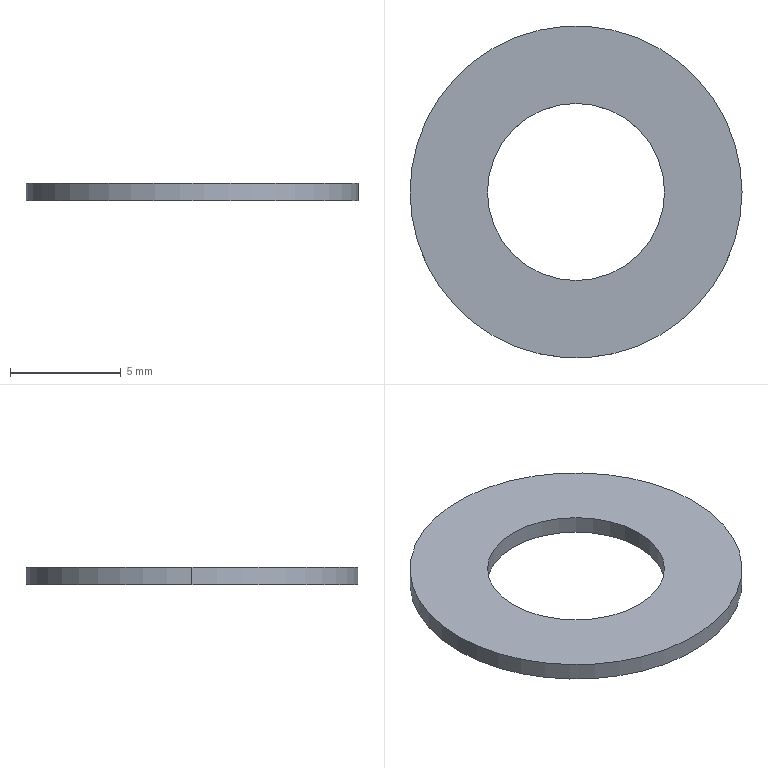Part | STEP file | E2E_X2D1_N_WASHER | 1 solid | 6 faces | box 15 x 15 x 0.8 mm | volume 101.159 mm3 | cylinder 4 | plane 2 | commonest cylinder face diameters 8 x2 15 x2
STEP:
#1=CARTESIAN_POINT('',(0.,0.,0.));
#2=DIRECTION('',(0.,0.,1.));
#3=DIRECTION('',(1.,0.,0.));
#4=AXIS2_PLACEMENT_3D('',#1,#2,#3);
#5=CARTESIAN_POINT('',(4.,0.,-0.8));
#6=VERTEX_POINT('',#5);
#7=CARTESIAN_POINT('',(4.,0.,0.));
#8=VERTEX_POINT('',#7);
#9=CARTESIAN_POINT('',(4.,0.,-0.8));
#10=DIRECTION('',(0.,0.,1.));
#11=VECTOR('',#10,1.);
#12=LINE('',#9,#11);
#13=CARTESIAN_POINT('',(0.,0.,-0.8));
#14=DIRECTION('',(0.,0.,1.));
#15=DIRECTION('',(1.,0.,0.));
#16=AXIS2_PLACEMENT_3D('',#13,#14,#15);
#17=CYLINDRICAL_SURFACE('',#16,4.);
#18=CARTESIAN_POINT('',(6.283,0.));
#19=DIRECTION('',(0.,1.));
#20=VECTOR('',#19,1.);
#21=LINE('',#18,#20);
#22=(GEOMETRIC_REPRESENTATION_CONTEXT(2)PARAMETRIC_REPRESENTATION_CONTEXT()REPRESENTATION_CONTEXT('',''));
#23=DEFINITIONAL_REPRESENTATION('',(#21),#22);
#24=PCURVE('',#17,#23);
#25=CARTESIAN_POINT('',(0.,0.,-0.8));
#26=DIRECTION('',(0.,0.,1.));
#27=DIRECTION('',(1.,0.,0.));
#28=AXIS2_PLACEMENT_3D('',#25,#26,#27);
#29=CYLINDRICAL_SURFACE('',#28,4.);
#30=CARTESIAN_POINT('',(0.,0.));
#31=DIRECTION('',(0.,1.));
#32=VECTOR('',#31,1.);
#33=LINE('',#30,#32);
#34=(GEOMETRIC_REPRESENTATION_CONTEXT(2)PARAMETRIC_REPRESENTATION_CONTEXT()REPRESENTATION_CONTEXT('',''));
#35=DEFINITIONAL_REPRESENTATION('',(#33),#34);
#36=PCURVE('',#29,#35);
#37=SURFACE_CURVE('',#12,(#24,#36),.PCURVE_S1.);
#38=EDGE_CURVE('',#6,#8,#37,.T.);
#39=ORIENTED_EDGE('',*,*,#38,.T.);
#40=CARTESIAN_POINT('',(-4.,0.,0.));
#41=VERTEX_POINT('',#40);
#42=CARTESIAN_POINT('',(0.,0.,0.));
#43=DIRECTION('',(0.,0.,1.));
#44=DIRECTION('',(1.,0.,0.));
#45=AXIS2_PLACEMENT_3D('',#42,#43,#44);
#46=CIRCLE('',#45,4.);
#47=CARTESIAN_POINT('',(0.,0.8));
#48=DIRECTION('',(1.,0.));
#49=VECTOR('',#48,1.);
#50=LINE('',#47,#49);
#51=(GEOMETRIC_REPRESENTATION_CONTEXT(2)PARAMETRIC_REPRESENTATION_CONTEXT()REPRESENTATION_CONTEXT('',''));
#52=DEFINITIONAL_REPRESENTATION('',(#50),#51);
#53=PCURVE('',#17,#52);
#54=CARTESIAN_POINT('',(0.,0.,0.));
#55=DIRECTION('',(0.,0.,1.));
#56=DIRECTION('',(1.,0.,0.));
#57=AXIS2_PLACEMENT_3D('',#54,#55,#56);
#58=PLANE('',#57);
#59=CARTESIAN_POINT('',(0.,0.));
#60=DIRECTION('',(1.,0.));
#61=AXIS2_PLACEMENT_2D('',#59,#60);
#62=CIRCLE('',#61,4.);
#63=(GEOMETRIC_REPRESENTATION_CONTEXT(2)PARAMETRIC_REPRESENTATION_CONTEXT()REPRESENTATION_CONTEXT('',''));
#64=DEFINITIONAL_REPRESENTATION('',(#62),#63);
#65=PCURVE('',#58,#64);
#66=SURFACE_CURVE('',#46,(#53,#65),.PCURVE_S1.);
#67=EDGE_CURVE('',#41,#8,#66,.T.);
#68=ORIENTED_EDGE('',*,*,#67,.F.);
#69=CARTESIAN_POINT('',(-4.,0.,-0.8));
#70=VERTEX_POINT('',#69);
#71=CARTESIAN_POINT('',(-4.,0.,-0.8));
#72=DIRECTION('',(0.,0.,1.));
#73=VECTOR('',#72,1.);
#74=LINE('',#71,#73);
#75=CARTESIAN_POINT('',(3.142,0.));
#76=DIRECTION('',(0.,1.));
#77=VECTOR('',#76,1.);
#78=LINE('',#75,#77);
#79=(GEOMETRIC_REPRESENTATION_CONTEXT(2)PARAMETRIC_REPRESENTATION_CONTEXT()REPRESENTATION_CONTEXT('',''));
#80=DEFINITIONAL_REPRESENTATION('',(#78),#79);
#81=PCURVE('',#17,#80);
#82=CARTESIAN_POINT('',(3.142,0.));
#83=DIRECTION('',(0.,1.));
#84=VECTOR('',#83,1.);
#85=LINE('',#82,#84);
#86=(GEOMETRIC_REPRESENTATION_CONTEXT(2)PARAMETRIC_REPRESENTATION_CONTEXT()REPRESENTATION_CONTEXT('',''));
#87=DEFINITIONAL_REPRESENTATION('',(#85),#86);
#88=PCURVE('',#29,#87);
#89=SURFACE_CURVE('',#74,(#81,#88),.PCURVE_S1.);
#90=EDGE_CURVE('',#70,#41,#89,.T.);
#91=ORIENTED_EDGE('',*,*,#90,.F.);
#92=CARTESIAN_POINT('',(0.,0.,-0.8));
#93=DIRECTION('',(0.,0.,1.));
#94=DIRECTION('',(1.,0.,0.));
#95=AXIS2_PLACEMENT_3D('',#92,#93,#94);
#96=CIRCLE('',#95,4.);
#97=CARTESIAN_POINT('',(0.,0.));
#98=DIRECTION('',(1.,0.));
#99=VECTOR('',#98,1.);
#100=LINE('',#97,#99);
#101=(GEOMETRIC_REPRESENTATION_CONTEXT(2)PARAMETRIC_REPRESENTATION_CONTEXT()REPRESENTATION_CONTEXT('',''));
#102=DEFINITIONAL_REPRESENTATION('',(#100),#101);
#103=PCURVE('',#17,#102);
#104=CARTESIAN_POINT('',(0.,0.,-0.8));
#105=DIRECTION('',(0.,0.,1.));
#106=DIRECTION('',(1.,0.,0.));
#107=AXIS2_PLACEMENT_3D('',#104,#105,#106);
#108=PLANE('',#107);
#109=CARTESIAN_POINT('',(0.,0.));
#110=DIRECTION('',(1.,0.));
#111=AXIS2_PLACEMENT_2D('',#109,#110);
#112=CIRCLE('',#111,4.);
#113=(GEOMETRIC_REPRESENTATION_CONTEXT(2)PARAMETRIC_REPRESENTATION_CONTEXT()REPRESENTATION_CONTEXT('',''));
#114=DEFINITIONAL_REPRESENTATION('',(#112),#113);
#115=PCURVE('',#108,#114);
#116=SURFACE_CURVE('',#96,(#103,#115),.PCURVE_S1.);
#117=EDGE_CURVE('',#70,#6,#116,.T.);
#118=ORIENTED_EDGE('',*,*,#117,.T.);
#119=EDGE_LOOP('',(#39,#68,#91,#118));
#120=FACE_BOUND('',#119,.F.);
#121=ADVANCED_FACE('',(#120),#17,.F.);
#122=CARTESIAN_POINT('',(7.5,0.,-0.8));
#123=VERTEX_POINT('',#122);
#124=CARTESIAN_POINT('',(-7.5,0.,-0.8));
#125=VERTEX_POINT('',#124);
#126=CARTESIAN_POINT('',(0.,0.,-0.8));
#127=DIRECTION('',(0.,0.,1.));
#128=DIRECTION('',(1.,0.,0.));
#129=AXIS2_PLACEMENT_3D('',#126,#127,#128);
#130=CIRCLE('',#129,7.5);
#131=CARTESIAN_POINT('',(0.,0.,-0.8));
#132=DIRECTION('',(0.,0.,1.));
#133=DIRECTION('',(1.,0.,0.));
#134=AXIS2_PLACEMENT_3D('',#131,#132,#133);
#135=CYLINDRICAL_SURFACE('',#134,7.5);
#136=CARTESIAN_POINT('',(0.,0.));
#137=DIRECTION('',(1.,0.));
#138=VECTOR('',#137,1.);
#139=LINE('',#136,#138);
#140=(GEOMETRIC_REPRESENTATION_CONTEXT(2)PARAMETRIC_REPRESENTATION_CONTEXT()REPRESENTATION_CONTEXT('',''));
#141=DEFINITIONAL_REPRESENTATION('',(#139),#140);
#142=PCURVE('',#135,#141);
#143=CARTESIAN_POINT('',(0.,0.));
#144=DIRECTION('',(1.,0.));
#145=AXIS2_PLACEMENT_2D('',#143,#144);
#146=CIRCLE('',#145,7.5);
#147=(GEOMETRIC_REPRESENTATION_CONTEXT(2)PARAMETRIC_REPRESENTATION_CONTEXT()REPRESENTATION_CONTEXT('',''));
#148=DEFINITIONAL_REPRESENTATION('',(#146),#147);
#149=PCURVE('',#108,#148);
#150=SURFACE_CURVE('',#130,(#142,#149),.PCURVE_S1.);
#151=EDGE_CURVE('',#123,#125,#150,.T.);
#152=ORIENTED_EDGE('',*,*,#151,.T.);
#153=CARTESIAN_POINT('',(-7.5,0.,0.));
#154=VERTEX_POINT('',#153);
#155=CARTESIAN_POINT('',(-7.5,0.,-0.8));
#156=DIRECTION('',(0.,0.,1.));
#157=VECTOR('',#156,1.);
#158=LINE('',#155,#157);
#159=CARTESIAN_POINT('',(3.142,0.));
#160=DIRECTION('',(0.,1.));
#161=VECTOR('',#160,1.);
#162=LINE('',#159,#161);
#163=(GEOMETRIC_REPRESENTATION_CONTEXT(2)PARAMETRIC_REPRESENTATION_CONTEXT()REPRESENTATION_CONTEXT('',''));
#164=DEFINITIONAL_REPRESENTATION('',(#162),#163);
#165=PCURVE('',#135,#164);
#166=CARTESIAN_POINT('',(0.,0.,-0.8));
#167=DIRECTION('',(0.,0.,1.));
#168=DIRECTION('',(1.,0.,0.));
#169=AXIS2_PLACEMENT_3D('',#166,#167,#168);
#170=CYLINDRICAL_SURFACE('',#169,7.5);
#171=CARTESIAN_POINT('',(3.142,0.));
#172=DIRECTION('',(0.,1.));
#173=VECTOR('',#172,1.);
#174=LINE('',#171,#173);
#175=(GEOMETRIC_REPRESENTATION_CONTEXT(2)PARAMETRIC_REPRESENTATION_CONTEXT()REPRESENTATION_CONTEXT('',''));
#176=DEFINITIONAL_REPRESENTATION('',(#174),#175);
#177=PCURVE('',#170,#176);
#178=SURFACE_CURVE('',#158,(#165,#177),.PCURVE_S1.);
#179=EDGE_CURVE('',#125,#154,#178,.T.);
#180=ORIENTED_EDGE('',*,*,#179,.T.);
#181=CARTESIAN_POINT('',(7.5,0.,0.));
#182=VERTEX_POINT('',#181);
#183=CARTESIAN_POINT('',(0.,0.,0.));
#184=DIRECTION('',(0.,0.,1.));
#185=DIRECTION('',(1.,0.,0.));
#186=AXIS2_PLACEMENT_3D('',#183,#184,#185);
#187=CIRCLE('',#186,7.5);
#188=CARTESIAN_POINT('',(0.,0.8));
#189=DIRECTION('',(1.,0.));
#190=VECTOR('',#189,1.);
#191=LINE('',#188,#190);
#192=(GEOMETRIC_REPRESENTATION_CONTEXT(2)PARAMETRIC_REPRESENTATION_CONTEXT()REPRESENTATION_CONTEXT('',''));
#193=DEFINITIONAL_REPRESENTATION('',(#191),#192);
#194=PCURVE('',#135,#193);
#195=CARTESIAN_POINT('',(0.,0.));
#196=DIRECTION('',(1.,0.));
#197=AXIS2_PLACEMENT_2D('',#195,#196);
#198=CIRCLE('',#197,7.5);
#199=(GEOMETRIC_REPRESENTATION_CONTEXT(2)PARAMETRIC_REPRESENTATION_CONTEXT()REPRESENTATION_CONTEXT('',''));
#200=DEFINITIONAL_REPRESENTATION('',(#198),#199);
#201=PCURVE('',#58,#200);
#202=SURFACE_CURVE('',#187,(#194,#201),.PCURVE_S1.);
#203=EDGE_CURVE('',#182,#154,#202,.T.);
#204=ORIENTED_EDGE('',*,*,#203,.F.);
#205=CARTESIAN_POINT('',(7.5,0.,-0.8));
#206=DIRECTION('',(0.,0.,1.));
#207=VECTOR('',#206,1.);
#208=LINE('',#205,#207);
#209=CARTESIAN_POINT('',(0.,0.));
#210=DIRECTION('',(0.,1.));
#211=VECTOR('',#210,1.);
#212=LINE('',#209,#211);
#213=(GEOMETRIC_REPRESENTATION_CONTEXT(2)PARAMETRIC_REPRESENTATION_CONTEXT()REPRESENTATION_CONTEXT('',''));
#214=DEFINITIONAL_REPRESENTATION('',(#212),#213);
#215=PCURVE('',#135,#214);
#216=CARTESIAN_POINT('',(6.283,0.));
#217=DIRECTION('',(0.,1.));
#218=VECTOR('',#217,1.);
#219=LINE('',#216,#218);
#220=(GEOMETRIC_REPRESENTATION_CONTEXT(2)PARAMETRIC_REPRESENTATION_CONTEXT()REPRESENTATION_CONTEXT('',''));
#221=DEFINITIONAL_REPRESENTATION('',(#219),#220);
#222=PCURVE('',#170,#221);
#223=SURFACE_CURVE('',#208,(#215,#222),.PCURVE_S1.);
#224=EDGE_CURVE('',#123,#182,#223,.T.);
#225=ORIENTED_EDGE('',*,*,#224,.F.);
#226=EDGE_LOOP('',(#152,#180,#204,#225));
#227=FACE_BOUND('',#226,.T.);
#228=ADVANCED_FACE('',(#227),#135,.T.);
#229=ORIENTED_EDGE('',*,*,#179,.F.);
#230=CARTESIAN_POINT('',(0.,0.,-0.8));
#231=DIRECTION('',(0.,0.,1.));
#232=DIRECTION('',(1.,0.,0.));
#233=AXIS2_PLACEMENT_3D('',#230,#231,#232);
#234=CIRCLE('',#233,7.5);
#235=CARTESIAN_POINT('',(0.,0.));
#236=DIRECTION('',(1.,0.));
#237=VECTOR('',#236,1.);
#238=LINE('',#235,#237);
#239=(GEOMETRIC_REPRESENTATION_CONTEXT(2)PARAMETRIC_REPRESENTATION_CONTEXT()REPRESENTATION_CONTEXT('',''));
#240=DEFINITIONAL_REPRESENTATION('',(#238),#239);
#241=PCURVE('',#170,#240);
#242=CARTESIAN_POINT('',(0.,0.));
#243=DIRECTION('',(1.,0.));
#244=AXIS2_PLACEMENT_2D('',#242,#243);
#245=CIRCLE('',#244,7.5);
#246=(GEOMETRIC_REPRESENTATION_CONTEXT(2)PARAMETRIC_REPRESENTATION_CONTEXT()REPRESENTATION_CONTEXT('',''));
#247=DEFINITIONAL_REPRESENTATION('',(#245),#246);
#248=PCURVE('',#108,#247);
#249=SURFACE_CURVE('',#234,(#241,#248),.PCURVE_S1.);
#250=EDGE_CURVE('',#125,#123,#249,.T.);
#251=ORIENTED_EDGE('',*,*,#250,.T.);
#252=ORIENTED_EDGE('',*,*,#224,.T.);
#253=CARTESIAN_POINT('',(0.,0.,0.));
#254=DIRECTION('',(0.,0.,1.));
#255=DIRECTION('',(1.,0.,0.));
#256=AXIS2_PLACEMENT_3D('',#253,#254,#255);
#257=CIRCLE('',#256,7.5);
#258=CARTESIAN_POINT('',(0.,0.8));
#259=DIRECTION('',(1.,0.));
#260=VECTOR('',#259,1.);
#261=LINE('',#258,#260);
#262=(GEOMETRIC_REPRESENTATION_CONTEXT(2)PARAMETRIC_REPRESENTATION_CONTEXT()REPRESENTATION_CONTEXT('',''));
#263=DEFINITIONAL_REPRESENTATION('',(#261),#262);
#264=PCURVE('',#170,#263);
#265=CARTESIAN_POINT('',(0.,0.));
#266=DIRECTION('',(1.,0.));
#267=AXIS2_PLACEMENT_2D('',#265,#266);
#268=CIRCLE('',#267,7.5);
#269=(GEOMETRIC_REPRESENTATION_CONTEXT(2)PARAMETRIC_REPRESENTATION_CONTEXT()REPRESENTATION_CONTEXT('',''));
#270=DEFINITIONAL_REPRESENTATION('',(#268),#269);
#271=PCURVE('',#58,#270);
#272=SURFACE_CURVE('',#257,(#264,#271),.PCURVE_S1.);
#273=EDGE_CURVE('',#154,#182,#272,.T.);
#274=ORIENTED_EDGE('',*,*,#273,.F.);
#275=EDGE_LOOP('',(#229,#251,#252,#274));
#276=FACE_BOUND('',#275,.T.);
#277=ADVANCED_FACE('',(#276),#170,.T.);
#278=CARTESIAN_POINT('',(0.,0.,-0.8));
#279=DIRECTION('',(0.,0.,1.));
#280=DIRECTION('',(1.,0.,0.));
#281=AXIS2_PLACEMENT_3D('',#278,#279,#280);
#282=CIRCLE('',#281,4.);
#283=CARTESIAN_POINT('',(0.,0.));
#284=DIRECTION('',(1.,0.));
#285=AXIS2_PLACEMENT_2D('',#283,#284);
#286=CIRCLE('',#285,4.);
#287=(GEOMETRIC_REPRESENTATION_CONTEXT(2)PARAMETRIC_REPRESENTATION_CONTEXT()REPRESENTATION_CONTEXT('',''));
#288=DEFINITIONAL_REPRESENTATION('',(#286),#287);
#289=PCURVE('',#108,#288);
#290=CARTESIAN_POINT('',(0.,0.));
#291=DIRECTION('',(1.,0.));
#292=VECTOR('',#291,1.);
#293=LINE('',#290,#292);
#294=(GEOMETRIC_REPRESENTATION_CONTEXT(2)PARAMETRIC_REPRESENTATION_CONTEXT()REPRESENTATION_CONTEXT('',''));
#295=DEFINITIONAL_REPRESENTATION('',(#293),#294);
#296=PCURVE('',#29,#295);
#297=SURFACE_CURVE('',#282,(#289,#296),.PCURVE_S1.);
#298=EDGE_CURVE('',#6,#70,#297,.T.);
#299=ORIENTED_EDGE('',*,*,#298,.T.);
#300=ORIENTED_EDGE('',*,*,#117,.T.);
#301=EDGE_LOOP('',(#299,#300));
#302=FACE_BOUND('',#301,.T.);
#303=ORIENTED_EDGE('',*,*,#151,.F.);
#304=ORIENTED_EDGE('',*,*,#250,.F.);
#305=EDGE_LOOP('',(#303,#304));
#306=FACE_BOUND('',#305,.T.);
#307=ADVANCED_FACE('',(#302,#306),#108,.F.);
#308=CARTESIAN_POINT('',(0.,0.,0.));
#309=DIRECTION('',(0.,0.,1.));
#310=DIRECTION('',(1.,0.,0.));
#311=AXIS2_PLACEMENT_3D('',#308,#309,#310);
#312=CIRCLE('',#311,4.);
#313=CARTESIAN_POINT('',(0.,0.));
#314=DIRECTION('',(1.,0.));
#315=AXIS2_PLACEMENT_2D('',#313,#314);
#316=CIRCLE('',#315,4.);
#317=(GEOMETRIC_REPRESENTATION_CONTEXT(2)PARAMETRIC_REPRESENTATION_CONTEXT()REPRESENTATION_CONTEXT('',''));
#318=DEFINITIONAL_REPRESENTATION('',(#316),#317);
#319=PCURVE('',#58,#318);
#320=CARTESIAN_POINT('',(0.,0.8));
#321=DIRECTION('',(1.,0.));
#322=VECTOR('',#321,1.);
#323=LINE('',#320,#322);
#324=(GEOMETRIC_REPRESENTATION_CONTEXT(2)PARAMETRIC_REPRESENTATION_CONTEXT()REPRESENTATION_CONTEXT('',''));
#325=DEFINITIONAL_REPRESENTATION('',(#323),#324);
#326=PCURVE('',#29,#325);
#327=SURFACE_CURVE('',#312,(#319,#326),.PCURVE_S1.);
#328=EDGE_CURVE('',#8,#41,#327,.T.);
#329=ORIENTED_EDGE('',*,*,#328,.F.);
#330=ORIENTED_EDGE('',*,*,#67,.F.);
#331=EDGE_LOOP('',(#329,#330));
#332=FACE_BOUND('',#331,.T.);
#333=ORIENTED_EDGE('',*,*,#203,.T.);
#334=ORIENTED_EDGE('',*,*,#273,.T.);
#335=EDGE_LOOP('',(#333,#334));
#336=FACE_BOUND('',#335,.T.);
#337=ADVANCED_FACE('',(#332,#336),#58,.T.);
#338=ORIENTED_EDGE('',*,*,#328,.F.);
#339=ORIENTED_EDGE('',*,*,#38,.F.);
#340=ORIENTED_EDGE('',*,*,#298,.T.);
#341=ORIENTED_EDGE('',*,*,#90,.T.);
#342=EDGE_LOOP('',(#338,#339,#340,#341));
#343=FACE_BOUND('',#342,.F.);
#344=ADVANCED_FACE('',(#343),#29,.F.);
#345=CLOSED_SHELL('',(#121,#228,#277,#307,#337,#344));
#346=MANIFOLD_SOLID_BREP('',#345);
#347=(LENGTH_UNIT()NAMED_UNIT(*)SI_UNIT(.MILLI.,.METRE.));
#348=UNCERTAINTY_MEASURE_WITH_UNIT(LENGTH_MEASURE(0.0000001),#347,'','');
#349=(NAMED_UNIT(*)PLANE_ANGLE_UNIT()SI_UNIT($,.RADIAN.));
#350=(NAMED_UNIT(*)SI_UNIT($,.STERADIAN.)SOLID_ANGLE_UNIT());
#351=(GEOMETRIC_REPRESENTATION_CONTEXT(3)GLOBAL_UNCERTAINTY_ASSIGNED_CONTEXT((#348))GLOBAL_UNIT_ASSIGNED_CONTEXT((#347,#349,#350))REPRESENTATION_CONTEXT('',''));
#352=ADVANCED_BREP_SHAPE_REPRESENTATION('',(#4,#346),#351);